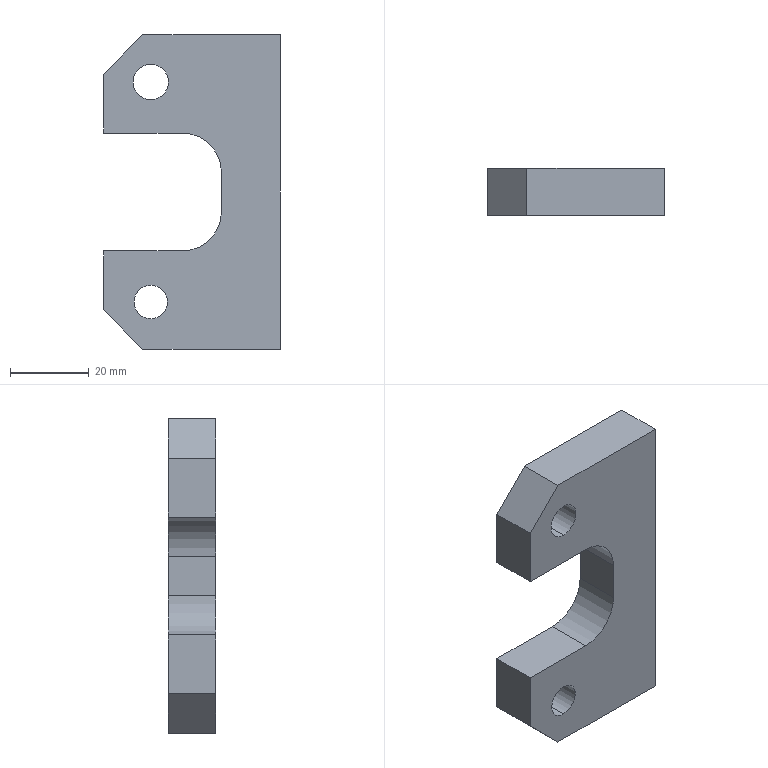Part | STEP file | PN_0048 | 1 solid | 26 faces | box 45 x 12 x 80 mm | volume 29583 mm3 | plane 12 | cylinder 10 | cone 4 | commonest cylinder face diameters 5 x4 8.5 x2 9 x2 20 x2